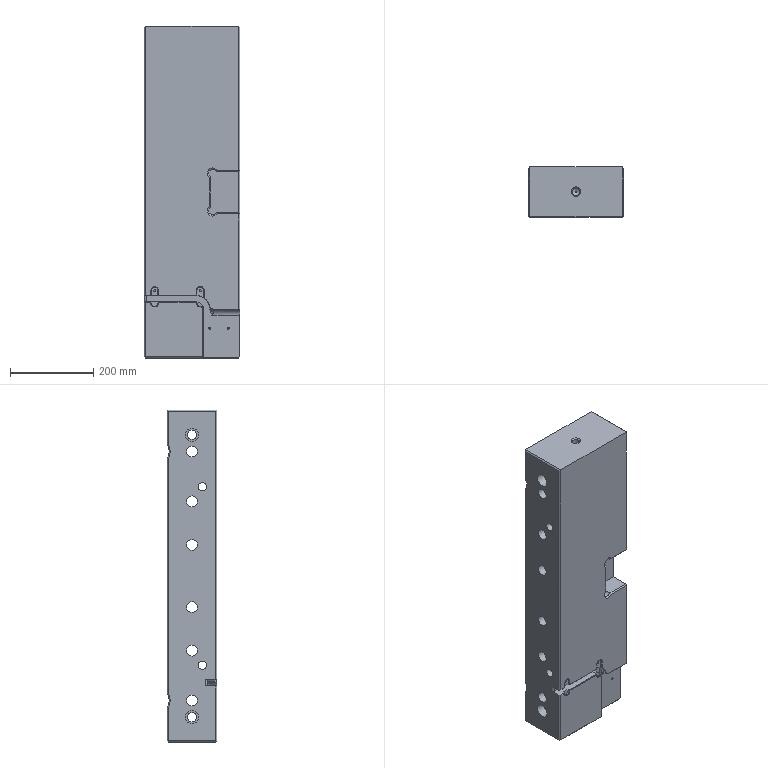Part | STEP file | solid 57 | 1 solid | 144 faces | box 230 x 120 x 800 mm | volume 20301168 mm3 | plane 84 | cylinder 36 | cone 23 | spline 1 | commonest cylinder face diameters 15 x8 26 x6 20 x5 4.2 x2 5 x2 10 x2